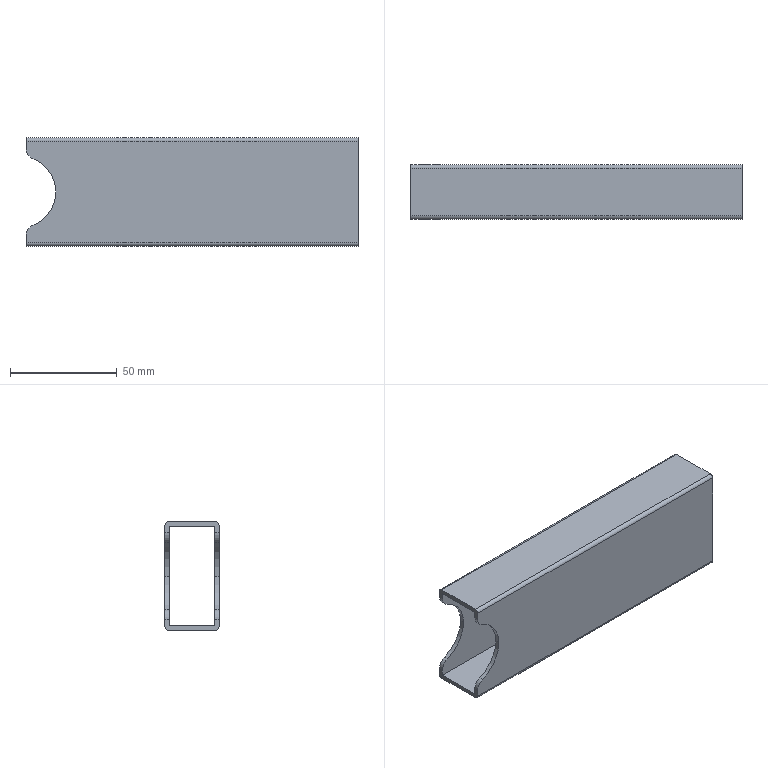Part | NX | features BREP 1 | 1 solid | 23 faces | box 155.702 x 25.4 x 50.8 mm | volume 42830 mm3 | cylinder 12 | plane 11 | commonest cylinder face diameters 3.175 x4 10.16 x4 33.528 x4
STEP:
#1=CARTESIAN_POINT('',(0.,12.7,-23.812));
#2=VERTEX_POINT('',#1);
#3=CARTESIAN_POINT('',(0.,12.7,-20.375));
#4=VERTEX_POINT('',#3);
#5=CARTESIAN_POINT('',(0.,12.7,-23.812));
#6=DIRECTION('',(0.,0.,1.));
#7=VECTOR('',#6,1000.);
#8=LINE('',#5,#7);
#9=EDGE_CURVE('',#2,#4,#8,.T.);
#10=ORIENTED_EDGE('',*,*,#9,.F.);
#11=CARTESIAN_POINT('',(0.,11.113,-25.4));
#12=VERTEX_POINT('',#11);
#13=CARTESIAN_POINT('',(0.,11.113,-23.812));
#14=DIRECTION('',(-1.,0.,0.));
#15=DIRECTION('',(0.,1.,0.));
#16=AXIS2_PLACEMENT_3D('',#13,#14,#15);
#17=CIRCLE('',#16,1.587);
#18=EDGE_CURVE('',#2,#12,#17,.T.);
#19=ORIENTED_EDGE('',*,*,#18,.T.);
#20=CARTESIAN_POINT('',(0.,-11.113,-25.4));
#21=VERTEX_POINT('',#20);
#22=CARTESIAN_POINT('',(0.,-11.113,-25.4));
#23=DIRECTION('',(0.,1.,0.));
#24=VECTOR('',#23,1000.);
#25=LINE('',#22,#24);
#26=EDGE_CURVE('',#21,#12,#25,.T.);
#27=ORIENTED_EDGE('',*,*,#26,.F.);
#28=CARTESIAN_POINT('',(0.,-12.7,-23.812));
#29=VERTEX_POINT('',#28);
#30=CARTESIAN_POINT('',(0.,-11.113,-23.812));
#31=DIRECTION('',(-1.,0.,0.));
#32=DIRECTION('',(0.,0.,-1.));
#33=AXIS2_PLACEMENT_3D('',#30,#31,#32);
#34=CIRCLE('',#33,1.587);
#35=EDGE_CURVE('',#21,#29,#34,.T.);
#36=ORIENTED_EDGE('',*,*,#35,.T.);
#37=CARTESIAN_POINT('',(0.,-12.7,-20.375));
#38=VERTEX_POINT('',#37);
#39=CARTESIAN_POINT('',(0.,-12.7,-20.375));
#40=DIRECTION('',(0.,0.,-1.));
#41=VECTOR('',#40,1000.);
#42=LINE('',#39,#41);
#43=EDGE_CURVE('',#38,#29,#42,.T.);
#44=ORIENTED_EDGE('',*,*,#43,.F.);
#45=CARTESIAN_POINT('',(0.,-10.719,-20.375));
#46=VERTEX_POINT('',#45);
#47=CARTESIAN_POINT('',(0.,-12.7,-20.375));
#48=DIRECTION('',(0.,1.,0.));
#49=VECTOR('',#48,1000.);
#50=LINE('',#47,#49);
#51=EDGE_CURVE('',#38,#46,#50,.T.);
#52=ORIENTED_EDGE('',*,*,#51,.T.);
#53=CARTESIAN_POINT('',(0.,-10.719,-23.419));
#54=VERTEX_POINT('',#53);
#55=CARTESIAN_POINT('',(0.,-10.719,-23.419));
#56=DIRECTION('',(0.,0.,1.));
#57=VECTOR('',#56,1000.);
#58=LINE('',#55,#57);
#59=EDGE_CURVE('',#54,#46,#58,.T.);
#60=ORIENTED_EDGE('',*,*,#59,.F.);
#61=CARTESIAN_POINT('',(0.,10.719,-23.419));
#62=VERTEX_POINT('',#61);
#63=CARTESIAN_POINT('',(0.,10.719,-23.419));
#64=DIRECTION('',(0.,-1.,0.));
#65=VECTOR('',#64,1000.);
#66=LINE('',#63,#65);
#67=EDGE_CURVE('',#62,#54,#66,.T.);
#68=ORIENTED_EDGE('',*,*,#67,.F.);
#69=CARTESIAN_POINT('',(0.,10.719,-20.375));
#70=VERTEX_POINT('',#69);
#71=CARTESIAN_POINT('',(0.,10.719,-20.375));
#72=DIRECTION('',(0.,0.,-1.));
#73=VECTOR('',#72,1000.);
#74=LINE('',#71,#73);
#75=EDGE_CURVE('',#70,#62,#74,.T.);
#76=ORIENTED_EDGE('',*,*,#75,.F.);
#77=CARTESIAN_POINT('',(0.,10.719,-20.375));
#78=DIRECTION('',(0.,1.,0.));
#79=VECTOR('',#78,1000.);
#80=LINE('',#77,#79);
#81=EDGE_CURVE('',#70,#4,#80,.T.);
#82=ORIENTED_EDGE('',*,*,#81,.T.);
#83=EDGE_LOOP('',(#10,#19,#27,#36,#44,#52,#60,#68,#76,#82));
#84=FACE_BOUND('',#83,.T.);
#85=CARTESIAN_POINT('',(0.,0.,0.));
#86=DIRECTION('',(1.,0.,0.));
#87=DIRECTION('',(0.,1.,0.));
#88=AXIS2_PLACEMENT_3D('',#85,#86,#87);
#89=PLANE('',#88);
#90=ADVANCED_FACE('',(#84),#89,.F.);
#91=CARTESIAN_POINT('',(0.,-12.7,23.812));
#92=VERTEX_POINT('',#91);
#93=CARTESIAN_POINT('',(0.,-12.7,20.375));
#94=VERTEX_POINT('',#93);
#95=CARTESIAN_POINT('',(0.,-12.7,23.812));
#96=DIRECTION('',(0.,0.,-1.));
#97=VECTOR('',#96,1000.);
#98=LINE('',#95,#97);
#99=EDGE_CURVE('',#92,#94,#98,.T.);
#100=ORIENTED_EDGE('',*,*,#99,.F.);
#101=CARTESIAN_POINT('',(0.,-11.113,25.4));
#102=VERTEX_POINT('',#101);
#103=CARTESIAN_POINT('',(0.,-11.113,23.812));
#104=DIRECTION('',(-1.,0.,0.));
#105=DIRECTION('',(0.,-1.,0.));
#106=AXIS2_PLACEMENT_3D('',#103,#104,#105);
#107=CIRCLE('',#106,1.587);
#108=EDGE_CURVE('',#92,#102,#107,.T.);
#109=ORIENTED_EDGE('',*,*,#108,.T.);
#110=CARTESIAN_POINT('',(0.,11.113,25.4));
#111=VERTEX_POINT('',#110);
#112=CARTESIAN_POINT('',(0.,11.113,25.4));
#113=DIRECTION('',(0.,-1.,0.));
#114=VECTOR('',#113,1000.);
#115=LINE('',#112,#114);
#116=EDGE_CURVE('',#111,#102,#115,.T.);
#117=ORIENTED_EDGE('',*,*,#116,.F.);
#118=CARTESIAN_POINT('',(0.,12.7,23.812));
#119=VERTEX_POINT('',#118);
#120=CARTESIAN_POINT('',(0.,11.113,23.812));
#121=DIRECTION('',(-1.,0.,0.));
#122=DIRECTION('',(0.,0.,1.));
#123=AXIS2_PLACEMENT_3D('',#120,#121,#122);
#124=CIRCLE('',#123,1.587);
#125=EDGE_CURVE('',#111,#119,#124,.T.);
#126=ORIENTED_EDGE('',*,*,#125,.T.);
#127=CARTESIAN_POINT('',(0.,12.7,20.375));
#128=VERTEX_POINT('',#127);
#129=CARTESIAN_POINT('',(0.,12.7,20.375));
#130=DIRECTION('',(0.,0.,1.));
#131=VECTOR('',#130,1000.);
#132=LINE('',#129,#131);
#133=EDGE_CURVE('',#128,#119,#132,.T.);
#134=ORIENTED_EDGE('',*,*,#133,.F.);
#135=CARTESIAN_POINT('',(0.,10.719,20.375));
#136=VERTEX_POINT('',#135);
#137=CARTESIAN_POINT('',(0.,12.7,20.375));
#138=DIRECTION('',(0.,-1.,0.));
#139=VECTOR('',#138,1000.);
#140=LINE('',#137,#139);
#141=EDGE_CURVE('',#128,#136,#140,.T.);
#142=ORIENTED_EDGE('',*,*,#141,.T.);
#143=CARTESIAN_POINT('',(0.,10.719,23.419));
#144=VERTEX_POINT('',#143);
#145=CARTESIAN_POINT('',(0.,10.719,23.419));
#146=DIRECTION('',(0.,0.,-1.));
#147=VECTOR('',#146,1000.);
#148=LINE('',#145,#147);
#149=EDGE_CURVE('',#144,#136,#148,.T.);
#150=ORIENTED_EDGE('',*,*,#149,.F.);
#151=CARTESIAN_POINT('',(0.,-10.719,23.419));
#152=VERTEX_POINT('',#151);
#153=CARTESIAN_POINT('',(0.,-10.719,23.419));
#154=DIRECTION('',(0.,1.,0.));
#155=VECTOR('',#154,1000.);
#156=LINE('',#153,#155);
#157=EDGE_CURVE('',#152,#144,#156,.T.);
#158=ORIENTED_EDGE('',*,*,#157,.F.);
#159=CARTESIAN_POINT('',(0.,-10.719,20.375));
#160=VERTEX_POINT('',#159);
#161=CARTESIAN_POINT('',(0.,-10.719,20.375));
#162=DIRECTION('',(0.,0.,1.));
#163=VECTOR('',#162,1000.);
#164=LINE('',#161,#163);
#165=EDGE_CURVE('',#160,#152,#164,.T.);
#166=ORIENTED_EDGE('',*,*,#165,.F.);
#167=CARTESIAN_POINT('',(0.,-10.719,20.375));
#168=DIRECTION('',(0.,-1.,0.));
#169=VECTOR('',#168,1000.);
#170=LINE('',#167,#169);
#171=EDGE_CURVE('',#160,#94,#170,.T.);
#172=ORIENTED_EDGE('',*,*,#171,.T.);
#173=EDGE_LOOP('',(#100,#109,#117,#126,#134,#142,#150,#158,#166,#172));
#174=FACE_BOUND('',#173,.T.);
#175=CARTESIAN_POINT('',(0.,0.,0.));
#176=DIRECTION('',(1.,0.,0.));
#177=DIRECTION('',(0.,1.,0.));
#178=AXIS2_PLACEMENT_3D('',#175,#176,#177);
#179=PLANE('',#178);
#180=ADVANCED_FACE('',(#174),#179,.F.);
#181=CARTESIAN_POINT('',(3.249,10.719,-15.637));
#182=VERTEX_POINT('',#181);
#183=CARTESIAN_POINT('',(5.08,10.719,-20.375));
#184=DIRECTION('',(0.,-1.,0.));
#185=DIRECTION('',(-0.3605,0.,0.9328));
#186=AXIS2_PLACEMENT_3D('',#183,#184,#185);
#187=CIRCLE('',#186,5.08);
#188=EDGE_CURVE('',#182,#70,#187,.T.);
#189=ORIENTED_EDGE('',*,*,#188,.F.);
#190=CARTESIAN_POINT('',(3.249,12.7,-15.637));
#191=VERTEX_POINT('',#190);
#192=CARTESIAN_POINT('',(3.249,10.719,-15.637));
#193=DIRECTION('',(0.,1.,0.));
#194=VECTOR('',#193,1000.);
#195=LINE('',#192,#194);
#196=EDGE_CURVE('',#182,#191,#195,.T.);
#197=ORIENTED_EDGE('',*,*,#196,.T.);
#198=CARTESIAN_POINT('',(5.08,12.7,-20.375));
#199=DIRECTION('',(0.,1.,0.));
#200=DIRECTION('',(-1.,0.,0.));
#201=AXIS2_PLACEMENT_3D('',#198,#199,#200);
#202=CIRCLE('',#201,5.08);
#203=EDGE_CURVE('',#4,#191,#202,.T.);
#204=ORIENTED_EDGE('',*,*,#203,.F.);
#205=ORIENTED_EDGE('',*,*,#81,.F.);
#206=EDGE_LOOP('',(#189,#197,#204,#205));
#207=FACE_BOUND('',#206,.T.);
#208=CARTESIAN_POINT('',(5.08,-12.922,-20.375));
#209=DIRECTION('',(0.,1.,0.));
#210=DIRECTION('',(-1.,0.,0.));
#211=AXIS2_PLACEMENT_3D('',#208,#209,#210);
#212=CYLINDRICAL_SURFACE('',#211,5.08);
#213=ADVANCED_FACE('',(#207),#212,.T.);
#214=CARTESIAN_POINT('',(3.249,12.7,15.637));
#215=VERTEX_POINT('',#214);
#216=CARTESIAN_POINT('',(13.97,12.7,0.));
#217=VERTEX_POINT('',#216);
#218=CARTESIAN_POINT('',(-2.794,12.7,0.));
#219=DIRECTION('',(0.,1.,0.));
#220=DIRECTION('',(0.3605,0.,0.9328));
#221=AXIS2_PLACEMENT_3D('',#218,#219,#220);
#222=CIRCLE('',#221,16.764);
#223=EDGE_CURVE('',#215,#217,#222,.T.);
#224=ORIENTED_EDGE('',*,*,#223,.F.);
#225=CARTESIAN_POINT('',(5.08,12.7,20.375));
#226=DIRECTION('',(0.,1.,0.));
#227=DIRECTION('',(-0.3605,0.,-0.9328));
#228=AXIS2_PLACEMENT_3D('',#225,#226,#227);
#229=CIRCLE('',#228,5.08);
#230=EDGE_CURVE('',#215,#128,#229,.T.);
#231=ORIENTED_EDGE('',*,*,#230,.T.);
#232=ORIENTED_EDGE('',*,*,#133,.T.);
#233=CARTESIAN_POINT('',(155.702,12.7,23.812));
#234=VERTEX_POINT('',#233);
#235=CARTESIAN_POINT('',(155.702,12.7,23.812));
#236=DIRECTION('',(-1.,0.,0.));
#237=VECTOR('',#236,1000.);
#238=LINE('',#235,#237);
#239=EDGE_CURVE('',#234,#119,#238,.T.);
#240=ORIENTED_EDGE('',*,*,#239,.F.);
#241=CARTESIAN_POINT('',(155.702,12.7,-23.812));
#242=VERTEX_POINT('',#241);
#243=CARTESIAN_POINT('',(155.702,12.7,-23.812));
#244=DIRECTION('',(0.,0.,1.));
#245=VECTOR('',#244,1000.);
#246=LINE('',#243,#245);
#247=EDGE_CURVE('',#242,#234,#246,.T.);
#248=ORIENTED_EDGE('',*,*,#247,.F.);
#249=CARTESIAN_POINT('',(155.702,12.7,-23.812));
#250=DIRECTION('',(-1.,0.,0.));
#251=VECTOR('',#250,1000.);
#252=LINE('',#249,#251);
#253=EDGE_CURVE('',#242,#2,#252,.T.);
#254=ORIENTED_EDGE('',*,*,#253,.T.);
#255=ORIENTED_EDGE('',*,*,#9,.T.);
#256=ORIENTED_EDGE('',*,*,#203,.T.);
#257=CARTESIAN_POINT('',(-2.794,12.7,0.));
#258=DIRECTION('',(0.,1.,0.));
#259=DIRECTION('',(0.3605,0.,0.9328));
#260=AXIS2_PLACEMENT_3D('',#257,#258,#259);
#261=CIRCLE('',#260,16.764);
#262=EDGE_CURVE('',#217,#191,#261,.T.);
#263=ORIENTED_EDGE('',*,*,#262,.F.);
#264=EDGE_LOOP('',(#224,#231,#232,#240,#248,#254,#255,#256,#263));
#265=FACE_BOUND('',#264,.T.);
#266=CARTESIAN_POINT('',(0.,12.7,-25.4));
#267=DIRECTION('',(0.,1.,0.));
#268=DIRECTION('',(1.,0.,0.));
#269=AXIS2_PLACEMENT_3D('',#266,#267,#268);
#270=PLANE('',#269);
#271=ADVANCED_FACE('',(#265),#270,.T.);
#272=CARTESIAN_POINT('',(155.702,11.113,-25.4));
#273=VERTEX_POINT('',#272);
#274=CARTESIAN_POINT('',(155.702,11.113,-23.812));
#275=DIRECTION('',(1.,0.,0.));
#276=DIRECTION('',(0.,0.,-1.));
#277=AXIS2_PLACEMENT_3D('',#274,#275,#276);
#278=CIRCLE('',#277,1.587);
#279=EDGE_CURVE('',#273,#242,#278,.T.);
#280=ORIENTED_EDGE('',*,*,#279,.F.);
#281=CARTESIAN_POINT('',(155.702,11.113,-25.4));
#282=DIRECTION('',(-1.,0.,0.));
#283=VECTOR('',#282,1000.);
#284=LINE('',#281,#283);
#285=EDGE_CURVE('',#273,#12,#284,.T.);
#286=ORIENTED_EDGE('',*,*,#285,.T.);
#287=ORIENTED_EDGE('',*,*,#18,.F.);
#288=ORIENTED_EDGE('',*,*,#253,.F.);
#289=EDGE_LOOP('',(#280,#286,#287,#288));
#290=FACE_BOUND('',#289,.T.);
#291=CARTESIAN_POINT('',(155.961,11.113,-23.812));
#292=DIRECTION('',(-1.,0.,0.));
#293=DIRECTION('',(0.,1.,0.));
#294=AXIS2_PLACEMENT_3D('',#291,#292,#293);
#295=CYLINDRICAL_SURFACE('',#294,1.587);
#296=ADVANCED_FACE('',(#290),#295,.T.);
#297=CARTESIAN_POINT('',(155.702,-11.113,-25.4));
#298=VERTEX_POINT('',#297);
#299=CARTESIAN_POINT('',(155.702,-11.113,-25.4));
#300=DIRECTION('',(0.,1.,0.));
#301=VECTOR('',#300,1000.);
#302=LINE('',#299,#301);
#303=EDGE_CURVE('',#298,#273,#302,.T.);
#304=ORIENTED_EDGE('',*,*,#303,.F.);
#305=CARTESIAN_POINT('',(155.702,-11.113,-25.4));
#306=DIRECTION('',(-1.,0.,0.));
#307=VECTOR('',#306,1000.);
#308=LINE('',#305,#307);
#309=EDGE_CURVE('',#298,#21,#308,.T.);
#310=ORIENTED_EDGE('',*,*,#309,.T.);
#311=ORIENTED_EDGE('',*,*,#26,.T.);
#312=ORIENTED_EDGE('',*,*,#285,.F.);
#313=EDGE_LOOP('',(#304,#310,#311,#312));
#314=FACE_BOUND('',#313,.T.);
#315=CARTESIAN_POINT('',(0.,-12.7,-25.4));
#316=DIRECTION('',(0.,0.,-1.));
#317=DIRECTION('',(0.,-1.,0.));
#318=AXIS2_PLACEMENT_3D('',#315,#316,#317);
#319=PLANE('',#318);
#320=ADVANCED_FACE('',(#314),#319,.T.);
#321=CARTESIAN_POINT('',(155.702,-12.7,-23.812));
#322=VERTEX_POINT('',#321);
#323=CARTESIAN_POINT('',(155.702,-11.113,-23.812));
#324=DIRECTION('',(1.,0.,0.));
#325=DIRECTION('',(0.,-1.,0.));
#326=AXIS2_PLACEMENT_3D('',#323,#324,#325);
#327=CIRCLE('',#326,1.587);
#328=EDGE_CURVE('',#322,#298,#327,.T.);
#329=ORIENTED_EDGE('',*,*,#328,.F.);
#330=CARTESIAN_POINT('',(155.702,-12.7,-23.812));
#331=DIRECTION('',(-1.,0.,0.));
#332=VECTOR('',#331,1000.);
#333=LINE('',#330,#332);
#334=EDGE_CURVE('',#322,#29,#333,.T.);
#335=ORIENTED_EDGE('',*,*,#334,.T.);
#336=ORIENTED_EDGE('',*,*,#35,.F.);
#337=ORIENTED_EDGE('',*,*,#309,.F.);
#338=EDGE_LOOP('',(#329,#335,#336,#337));
#339=FACE_BOUND('',#338,.T.);
#340=CARTESIAN_POINT('',(155.961,-11.113,-23.812));
#341=DIRECTION('',(-1.,0.,0.));
#342=DIRECTION('',(0.,0.,-1.));
#343=AXIS2_PLACEMENT_3D('',#340,#341,#342);
#344=CYLINDRICAL_SURFACE('',#343,1.587);
#345=ADVANCED_FACE('',(#339),#344,.T.);
#346=ORIENTED_EDGE('',*,*,#43,.T.);
#347=ORIENTED_EDGE('',*,*,#334,.F.);
#348=CARTESIAN_POINT('',(155.702,-12.7,23.812));
#349=VERTEX_POINT('',#348);
#350=CARTESIAN_POINT('',(155.702,-12.7,23.812));
#351=DIRECTION('',(0.,0.,-1.));
#352=VECTOR('',#351,1000.);
#353=LINE('',#350,#352);
#354=EDGE_CURVE('',#349,#322,#353,.T.);
#355=ORIENTED_EDGE('',*,*,#354,.F.);
#356=CARTESIAN_POINT('',(155.702,-12.7,23.812));
#357=DIRECTION('',(-1.,0.,0.));
#358=VECTOR('',#357,1000.);
#359=LINE('',#356,#358);
#360=EDGE_CURVE('',#349,#92,#359,.T.);
#361=ORIENTED_EDGE('',*,*,#360,.T.);
#362=ORIENTED_EDGE('',*,*,#99,.T.);
#363=CARTESIAN_POINT('',(3.249,-12.7,15.637));
#364=VERTEX_POINT('',#363);
#365=CARTESIAN_POINT('',(5.08,-12.7,20.375));
#366=DIRECTION('',(0.,-1.,0.));
#367=DIRECTION('',(-1.,0.,0.));
#368=AXIS2_PLACEMENT_3D('',#365,#366,#367);
#369=CIRCLE('',#368,5.08);
#370=EDGE_CURVE('',#94,#364,#369,.T.);
#371=ORIENTED_EDGE('',*,*,#370,.T.);
#372=CARTESIAN_POINT('',(13.97,-12.7,0.));
#373=VERTEX_POINT('',#372);
#374=CARTESIAN_POINT('',(-2.794,-12.7,0.));
#375=DIRECTION('',(0.,1.,0.));
#376=DIRECTION('',(0.3605,0.,0.9328));
#377=AXIS2_PLACEMENT_3D('',#374,#375,#376);
#378=CIRCLE('',#377,16.764);
#379=EDGE_CURVE('',#364,#373,#378,.T.);
#380=ORIENTED_EDGE('',*,*,#379,.T.);
#381=CARTESIAN_POINT('',(3.249,-12.7,-15.637));
#382=VERTEX_POINT('',#381);
#383=CARTESIAN_POINT('',(-2.794,-12.7,0.));
#384=DIRECTION('',(0.,1.,0.));
#385=DIRECTION('',(0.3605,0.,0.9328));
#386=AXIS2_PLACEMENT_3D('',#383,#384,#385);
#387=CIRCLE('',#386,16.764);
#388=EDGE_CURVE('',#373,#382,#387,.T.);
#389=ORIENTED_EDGE('',*,*,#388,.T.);
#390=CARTESIAN_POINT('',(5.08,-12.7,-20.375));
#391=DIRECTION('',(0.,-1.,0.));
#392=DIRECTION('',(-0.3605,0.,0.9328));
#393=AXIS2_PLACEMENT_3D('',#390,#391,#392);
#394=CIRCLE('',#393,5.08);
#395=EDGE_CURVE('',#382,#38,#394,.T.);
#396=ORIENTED_EDGE('',*,*,#395,.T.);
#397=EDGE_LOOP('',(#346,#347,#355,#361,#362,#371,#380,#389,#396));
#398=FACE_BOUND('',#397,.T.);
#399=CARTESIAN_POINT('',(0.,-12.7,25.4));
#400=DIRECTION('',(0.,-1.,0.));
#401=DIRECTION('',(0.,0.,-1.));
#402=AXIS2_PLACEMENT_3D('',#399,#400,#401);
#403=PLANE('',#402);
#404=ADVANCED_FACE('',(#398),#403,.T.);
#405=ORIENTED_EDGE('',*,*,#395,.F.);
#406=CARTESIAN_POINT('',(3.249,-10.719,-15.637));
#407=VERTEX_POINT('',#406);
#408=CARTESIAN_POINT('',(3.249,-12.7,-15.637));
#409=DIRECTION('',(0.,1.,0.));
#410=VECTOR('',#409,1000.);
#411=LINE('',#408,#410);
#412=EDGE_CURVE('',#382,#407,#411,.T.);
#413=ORIENTED_EDGE('',*,*,#412,.T.);
#414=CARTESIAN_POINT('',(5.08,-10.719,-20.375));
#415=DIRECTION('',(0.,1.,0.));
#416=DIRECTION('',(-1.,0.,0.));
#417=AXIS2_PLACEMENT_3D('',#414,#415,#416);
#418=CIRCLE('',#417,5.08);
#419=EDGE_CURVE('',#46,#407,#418,.T.);
#420=ORIENTED_EDGE('',*,*,#419,.F.);
#421=ORIENTED_EDGE('',*,*,#51,.F.);
#422=EDGE_LOOP('',(#405,#413,#420,#421));
#423=FACE_BOUND('',#422,.T.);
#424=CARTESIAN_POINT('',(5.08,-12.922,-20.375));
#425=DIRECTION('',(0.,1.,0.));
#426=DIRECTION('',(-1.,0.,0.));
#427=AXIS2_PLACEMENT_3D('',#424,#425,#426);
#428=CYLINDRICAL_SURFACE('',#427,5.08);
#429=ADVANCED_FACE('',(#423),#428,.T.);
#430=CARTESIAN_POINT('',(3.249,-10.719,15.637));
#431=VERTEX_POINT('',#430);
#432=CARTESIAN_POINT('',(13.97,-10.719,0.));
#433=VERTEX_POINT('',#432);
#434=CARTESIAN_POINT('',(-2.794,-10.719,0.));
#435=DIRECTION('',(0.,1.,0.));
#436=DIRECTION('',(0.3605,0.,0.9328));
#437=AXIS2_PLACEMENT_3D('',#434,#435,#436);
#438=CIRCLE('',#437,16.764);
#439=EDGE_CURVE('',#431,#433,#438,.T.);
#440=ORIENTED_EDGE('',*,*,#439,.F.);
#441=CARTESIAN_POINT('',(5.08,-10.719,20.375));
#442=DIRECTION('',(0.,1.,0.));
#443=DIRECTION('',(-0.3605,0.,-0.9328));
#444=AXIS2_PLACEMENT_3D('',#441,#442,#443);
#445=CIRCLE('',#444,5.08);
#446=EDGE_CURVE('',#431,#160,#445,.T.);
#447=ORIENTED_EDGE('',*,*,#446,.T.);
#448=ORIENTED_EDGE('',*,*,#165,.T.);
#449=CARTESIAN_POINT('',(155.702,-10.719,23.419));
#450=VERTEX_POINT('',#449);
#451=CARTESIAN_POINT('',(0.,-10.719,23.419));
#452=DIRECTION('',(1.,0.,0.));
#453=VECTOR('',#452,1000.);
#454=LINE('',#451,#453);
#455=EDGE_CURVE('',#152,#450,#454,.T.);
#456=ORIENTED_EDGE('',*,*,#455,.T.);
#457=CARTESIAN_POINT('',(155.702,-10.719,-23.419));
#458=VERTEX_POINT('',#457);
#459=CARTESIAN_POINT('',(155.702,-10.719,-23.419));
#460=DIRECTION('',(0.,0.,1.));
#461=VECTOR('',#460,1000.);
#462=LINE('',#459,#461);
#463=EDGE_CURVE('',#458,#450,#462,.T.);
#464=ORIENTED_EDGE('',*,*,#463,.F.);
#465=CARTESIAN_POINT('',(0.,-10.719,-23.419));
#466=DIRECTION('',(1.,0.,0.));
#467=VECTOR('',#466,1000.);
#468=LINE('',#465,#467);
#469=EDGE_CURVE('',#54,#458,#468,.T.);
#470=ORIENTED_EDGE('',*,*,#469,.F.);
#471=ORIENTED_EDGE('',*,*,#59,.T.);
#472=ORIENTED_EDGE('',*,*,#419,.T.);
#473=CARTESIAN_POINT('',(-2.794,-10.719,0.));
#474=DIRECTION('',(0.,1.,0.));
#475=DIRECTION('',(0.3605,0.,0.9328));
#476=AXIS2_PLACEMENT_3D('',#473,#474,#475);
#477=CIRCLE('',#476,16.764);
#478=EDGE_CURVE('',#433,#407,#477,.T.);
#479=ORIENTED_EDGE('',*,*,#478,.F.);
#480=EDGE_LOOP('',(#440,#447,#448,#456,#464,#470,#471,#472,#479));
#481=FACE_BOUND('',#480,.T.);
#482=CARTESIAN_POINT('',(0.,-10.719,-23.419));
#483=DIRECTION('',(0.,1.,0.));
#484=DIRECTION('',(1.,0.,0.));
#485=AXIS2_PLACEMENT_3D('',#482,#483,#484);
#486=PLANE('',#485);
#487=ADVANCED_FACE('',(#481),#486,.T.);
#488=ORIENTED_EDGE('',*,*,#469,.T.);
#489=CARTESIAN_POINT('',(155.702,10.719,-23.419));
#490=VERTEX_POINT('',#489);
#491=CARTESIAN_POINT('',(155.702,10.719,-23.419));
#492=DIRECTION('',(0.,-1.,0.));
#493=VECTOR('',#492,1000.);
#494=LINE('',#491,#493);
#495=EDGE_CURVE('',#490,#458,#494,.T.);
#496=ORIENTED_EDGE('',*,*,#495,.F.);
#497=CARTESIAN_POINT('',(0.,10.719,-23.419));
#498=DIRECTION('',(1.,0.,0.));
#499=VECTOR('',#498,1000.);
#500=LINE('',#497,#499);
#501=EDGE_CURVE('',#62,#490,#500,.T.);
#502=ORIENTED_EDGE('',*,*,#501,.F.);
#503=ORIENTED_EDGE('',*,*,#67,.T.);
#504=EDGE_LOOP('',(#488,#496,#502,#503));
#505=FACE_BOUND('',#504,.T.);
#506=CARTESIAN_POINT('',(0.,10.719,-23.419));
#507=DIRECTION('',(0.,0.,1.));
#508=DIRECTION('',(1.,0.,0.));
#509=AXIS2_PLACEMENT_3D('',#506,#507,#508);
#510=PLANE('',#509);
#511=ADVANCED_FACE('',(#505),#510,.T.);
#512=ORIENTED_EDGE('',*,*,#75,.T.);
#513=ORIENTED_EDGE('',*,*,#501,.T.);
#514=CARTESIAN_POINT('',(155.702,10.719,23.419));
#515=VERTEX_POINT('',#514);
#516=CARTESIAN_POINT('',(155.702,10.719,23.419));
#517=DIRECTION('',(0.,0.,-1.));
#518=VECTOR('',#517,1000.);
#519=LINE('',#516,#518);
#520=EDGE_CURVE('',#515,#490,#519,.T.);
#521=ORIENTED_EDGE('',*,*,#520,.F.);
#522=CARTESIAN_POINT('',(0.,10.719,23.419));
#523=DIRECTION('',(1.,0.,0.));
#524=VECTOR('',#523,1000.);
#525=LINE('',#522,#524);
#526=EDGE_CURVE('',#144,#515,#525,.T.);
#527=ORIENTED_EDGE('',*,*,#526,.F.);
#528=ORIENTED_EDGE('',*,*,#149,.T.);
#529=CARTESIAN_POINT('',(3.249,10.719,15.637));
#530=VERTEX_POINT('',#529);
#531=CARTESIAN_POINT('',(5.08,10.719,20.375));
#532=DIRECTION('',(0.,-1.,0.));
#533=DIRECTION('',(-1.,0.,0.));
#534=AXIS2_PLACEMENT_3D('',#531,#532,#533);
#535=CIRCLE('',#534,5.08);
#536=EDGE_CURVE('',#136,#530,#535,.T.);
#537=ORIENTED_EDGE('',*,*,#536,.T.);
#538=CARTESIAN_POINT('',(13.97,10.719,0.));
#539=VERTEX_POINT('',#538);
#540=CARTESIAN_POINT('',(-2.794,10.719,0.));
#541=DIRECTION('',(0.,1.,0.));
#542=DIRECTION('',(0.3605,0.,0.9328));
#543=AXIS2_PLACEMENT_3D('',#540,#541,#542);
#544=CIRCLE('',#543,16.764);
#545=EDGE_CURVE('',#530,#539,#544,.T.);
#546=ORIENTED_EDGE('',*,*,#545,.T.);
#547=CARTESIAN_POINT('',(-2.794,10.719,0.));
#548=DIRECTION('',(0.,1.,0.));
#549=DIRECTION('',(0.3605,0.,0.9328));
#550=AXIS2_PLACEMENT_3D('',#547,#548,#549);
#551=CIRCLE('',#550,16.764);
#552=EDGE_CURVE('',#539,#182,#551,.T.);
#553=ORIENTED_EDGE('',*,*,#552,.T.);
#554=ORIENTED_EDGE('',*,*,#188,.T.);
#555=EDGE_LOOP('',(#512,#513,#521,#527,#528,#537,#546,#553,#554));
#556=FACE_BOUND('',#555,.T.);
#557=CARTESIAN_POINT('',(0.,10.719,23.419));
#558=DIRECTION('',(0.,-1.,0.));
#559=DIRECTION('',(0.,0.,-1.));
#560=AXIS2_PLACEMENT_3D('',#557,#558,#559);
#561=PLANE('',#560);
#562=ADVANCED_FACE('',(#556),#561,.T.);
#563=CARTESIAN_POINT('',(13.97,15.24,0.));
#564=DIRECTION('',(0.,1.,0.));
#565=VECTOR('',#564,1000.);
#566=LINE('',#563,#565);
#567=EDGE_CURVE('',#539,#217,#566,.T.);
#568=ORIENTED_EDGE('',*,*,#567,.F.);
#569=ORIENTED_EDGE('',*,*,#545,.F.);
#570=CARTESIAN_POINT('',(3.249,12.7,15.637));
#571=DIRECTION('',(0.,-1.,0.));
#572=VECTOR('',#571,1000.);
#573=LINE('',#570,#572);
#574=EDGE_CURVE('',#215,#530,#573,.T.);
#575=ORIENTED_EDGE('',*,*,#574,.F.);
#576=ORIENTED_EDGE('',*,*,#223,.T.);
#577=EDGE_LOOP('',(#568,#569,#575,#576));
#578=FACE_BOUND('',#577,.T.);
#579=CARTESIAN_POINT('',(-2.794,15.24,0.));
#580=DIRECTION('',(0.,1.,0.));
#581=DIRECTION('',(1.,0.,0.));
#582=AXIS2_PLACEMENT_3D('',#579,#580,#581);
#583=CYLINDRICAL_SURFACE('',#582,16.764);
#584=ADVANCED_FACE('',(#578),#583,.F.);
#585=CARTESIAN_POINT('',(13.97,15.24,0.));
#586=DIRECTION('',(0.,1.,0.));
#587=VECTOR('',#586,1000.);
#588=LINE('',#585,#587);
#589=EDGE_CURVE('',#373,#433,#588,.T.);
#590=ORIENTED_EDGE('',*,*,#589,.F.);
#591=ORIENTED_EDGE('',*,*,#379,.F.);
#592=CARTESIAN_POINT('',(3.249,-10.719,15.637));
#593=DIRECTION('',(0.,-1.,0.));
#594=VECTOR('',#593,1000.);
#595=LINE('',#592,#594);
#596=EDGE_CURVE('',#431,#364,#595,.T.);
#597=ORIENTED_EDGE('',*,*,#596,.F.);
#598=ORIENTED_EDGE('',*,*,#439,.T.);
#599=EDGE_LOOP('',(#590,#591,#597,#598));
#600=FACE_BOUND('',#599,.T.);
#601=CARTESIAN_POINT('',(-2.794,15.24,0.));
#602=DIRECTION('',(0.,1.,0.));
#603=DIRECTION('',(1.,0.,0.));
#604=AXIS2_PLACEMENT_3D('',#601,#602,#603);
#605=CYLINDRICAL_SURFACE('',#604,16.764);
#606=ADVANCED_FACE('',(#600),#605,.F.);
#607=ORIENTED_EDGE('',*,*,#230,.F.);
#608=ORIENTED_EDGE('',*,*,#574,.T.);
#609=ORIENTED_EDGE('',*,*,#536,.F.);
#610=ORIENTED_EDGE('',*,*,#141,.F.);
#611=EDGE_LOOP('',(#607,#608,#609,#610));
#612=FACE_BOUND('',#611,.T.);
#613=CARTESIAN_POINT('',(5.08,12.967,20.375));
#614=DIRECTION('',(0.,-1.,0.));
#615=DIRECTION('',(-1.,0.,0.));
#616=AXIS2_PLACEMENT_3D('',#613,#614,#615);
#617=CYLINDRICAL_SURFACE('',#616,5.08);
#618=ADVANCED_FACE('',(#612),#617,.T.);
#619=ORIENTED_EDGE('',*,*,#446,.F.);
#620=ORIENTED_EDGE('',*,*,#596,.T.);
#621=ORIENTED_EDGE('',*,*,#370,.F.);
#622=ORIENTED_EDGE('',*,*,#171,.F.);
#623=EDGE_LOOP('',(#619,#620,#621,#622));
#624=FACE_BOUND('',#623,.T.);
#625=CARTESIAN_POINT('',(5.08,12.967,20.375));
#626=DIRECTION('',(0.,-1.,0.));
#627=DIRECTION('',(-1.,0.,0.));
#628=AXIS2_PLACEMENT_3D('',#625,#626,#627);
#629=CYLINDRICAL_SURFACE('',#628,5.08);
#630=ADVANCED_FACE('',(#624),#629,.T.);
#631=ORIENTED_EDGE('',*,*,#526,.T.);
#632=CARTESIAN_POINT('',(155.702,-10.719,23.419));
#633=DIRECTION('',(0.,1.,0.));
#634=VECTOR('',#633,1000.);
#635=LINE('',#632,#634);
#636=EDGE_CURVE('',#450,#515,#635,.T.);
#637=ORIENTED_EDGE('',*,*,#636,.F.);
#638=ORIENTED_EDGE('',*,*,#455,.F.);
#639=ORIENTED_EDGE('',*,*,#157,.T.);
#640=EDGE_LOOP('',(#631,#637,#638,#639));
#641=FACE_BOUND('',#640,.T.);
#642=CARTESIAN_POINT('',(0.,-10.719,23.419));
#643=DIRECTION('',(0.,0.,-1.));
#644=DIRECTION('',(0.,-1.,0.));
#645=AXIS2_PLACEMENT_3D('',#642,#643,#644);
#646=PLANE('',#645);
#647=ADVANCED_FACE('',(#641),#646,.T.);
#648=CARTESIAN_POINT('',(155.702,11.113,25.4));
#649=VERTEX_POINT('',#648);
#650=CARTESIAN_POINT('',(155.702,-11.113,25.4));
#651=VERTEX_POINT('',#650);
#652=CARTESIAN_POINT('',(155.702,11.113,25.4));
#653=DIRECTION('',(0.,-1.,0.));
#654=VECTOR('',#653,1000.);
#655=LINE('',#652,#654);
#656=EDGE_CURVE('',#649,#651,#655,.T.);
#657=ORIENTED_EDGE('',*,*,#656,.T.);
#658=CARTESIAN_POINT('',(155.702,-11.113,23.812));
#659=DIRECTION('',(1.,0.,0.));
#660=DIRECTION('',(0.,0.,1.));
#661=AXIS2_PLACEMENT_3D('',#658,#659,#660);
#662=CIRCLE('',#661,1.587);
#663=EDGE_CURVE('',#651,#349,#662,.T.);
#664=ORIENTED_EDGE('',*,*,#663,.T.);
#665=ORIENTED_EDGE('',*,*,#354,.T.);
#666=ORIENTED_EDGE('',*,*,#328,.T.);
#667=ORIENTED_EDGE('',*,*,#303,.T.);
#668=ORIENTED_EDGE('',*,*,#279,.T.);
#669=ORIENTED_EDGE('',*,*,#247,.T.);
#670=CARTESIAN_POINT('',(155.702,11.113,23.812));
#671=DIRECTION('',(1.,0.,0.));
#672=DIRECTION('',(0.,1.,0.));
#673=AXIS2_PLACEMENT_3D('',#670,#671,#672);
#674=CIRCLE('',#673,1.587);
#675=EDGE_CURVE('',#234,#649,#674,.T.);
#676=ORIENTED_EDGE('',*,*,#675,.T.);
#677=EDGE_LOOP('',(#657,#664,#665,#666,#667,#668,#669,#676));
#678=FACE_BOUND('',#677,.T.);
#679=ORIENTED_EDGE('',*,*,#463,.T.);
#680=ORIENTED_EDGE('',*,*,#636,.T.);
#681=ORIENTED_EDGE('',*,*,#520,.T.);
#682=ORIENTED_EDGE('',*,*,#495,.T.);
#683=EDGE_LOOP('',(#679,#680,#681,#682));
#684=FACE_BOUND('',#683,.T.);
#685=CARTESIAN_POINT('',(155.702,0.,0.));
#686=DIRECTION('',(1.,0.,0.));
#687=DIRECTION('',(0.,1.,0.));
#688=AXIS2_PLACEMENT_3D('',#685,#686,#687);
#689=PLANE('',#688);
#690=ADVANCED_FACE('',(#678,#684),#689,.T.);
#691=ORIENTED_EDGE('',*,*,#675,.F.);
#692=ORIENTED_EDGE('',*,*,#239,.T.);
#693=ORIENTED_EDGE('',*,*,#125,.F.);
#694=CARTESIAN_POINT('',(155.702,11.113,25.4));
#695=DIRECTION('',(-1.,0.,0.));
#696=VECTOR('',#695,1000.);
#697=LINE('',#694,#696);
#698=EDGE_CURVE('',#649,#111,#697,.T.);
#699=ORIENTED_EDGE('',*,*,#698,.F.);
#700=EDGE_LOOP('',(#691,#692,#693,#699));
#701=FACE_BOUND('',#700,.T.);
#702=CARTESIAN_POINT('',(155.961,11.113,23.812));
#703=DIRECTION('',(-1.,0.,0.));
#704=DIRECTION('',(0.,0.,1.));
#705=AXIS2_PLACEMENT_3D('',#702,#703,#704);
#706=CYLINDRICAL_SURFACE('',#705,1.587);
#707=ADVANCED_FACE('',(#701),#706,.T.);
#708=ORIENTED_EDGE('',*,*,#116,.T.);
#709=CARTESIAN_POINT('',(155.702,-11.113,25.4));
#710=DIRECTION('',(-1.,0.,0.));
#711=VECTOR('',#710,1000.);
#712=LINE('',#709,#711);
#713=EDGE_CURVE('',#651,#102,#712,.T.);
#714=ORIENTED_EDGE('',*,*,#713,.F.);
#715=ORIENTED_EDGE('',*,*,#656,.F.);
#716=ORIENTED_EDGE('',*,*,#698,.T.);
#717=EDGE_LOOP('',(#708,#714,#715,#716));
#718=FACE_BOUND('',#717,.T.);
#719=CARTESIAN_POINT('',(0.,12.7,25.4));
#720=DIRECTION('',(0.,0.,1.));
#721=DIRECTION('',(1.,0.,0.));
#722=AXIS2_PLACEMENT_3D('',#719,#720,#721);
#723=PLANE('',#722);
#724=ADVANCED_FACE('',(#718),#723,.T.);
#725=ORIENTED_EDGE('',*,*,#663,.F.);
#726=ORIENTED_EDGE('',*,*,#713,.T.);
#727=ORIENTED_EDGE('',*,*,#108,.F.);
#728=ORIENTED_EDGE('',*,*,#360,.F.);
#729=EDGE_LOOP('',(#725,#726,#727,#728));
#730=FACE_BOUND('',#729,.T.);
#731=CARTESIAN_POINT('',(155.961,-11.113,23.812));
#732=DIRECTION('',(-1.,0.,0.));
#733=DIRECTION('',(0.,-1.,0.));
#734=AXIS2_PLACEMENT_3D('',#731,#732,#733);
#735=CYLINDRICAL_SURFACE('',#734,1.587);
#736=ADVANCED_FACE('',(#730),#735,.T.);
#737=ORIENTED_EDGE('',*,*,#388,.F.);
#738=ORIENTED_EDGE('',*,*,#589,.T.);
#739=ORIENTED_EDGE('',*,*,#478,.T.);
#740=ORIENTED_EDGE('',*,*,#412,.F.);
#741=EDGE_LOOP('',(#737,#738,#739,#740));
#742=FACE_BOUND('',#741,.T.);
#743=CARTESIAN_POINT('',(-2.794,15.24,0.));
#744=DIRECTION('',(0.,1.,0.));
#745=DIRECTION('',(1.,0.,0.));
#746=AXIS2_PLACEMENT_3D('',#743,#744,#745);
#747=CYLINDRICAL_SURFACE('',#746,16.764);
#748=ADVANCED_FACE('',(#742),#747,.F.);
#749=ORIENTED_EDGE('',*,*,#552,.F.);
#750=ORIENTED_EDGE('',*,*,#567,.T.);
#751=ORIENTED_EDGE('',*,*,#262,.T.);
#752=ORIENTED_EDGE('',*,*,#196,.F.);
#753=EDGE_LOOP('',(#749,#750,#751,#752));
#754=FACE_BOUND('',#753,.T.);
#755=CARTESIAN_POINT('',(-2.794,15.24,0.));
#756=DIRECTION('',(0.,1.,0.));
#757=DIRECTION('',(1.,0.,0.));
#758=AXIS2_PLACEMENT_3D('',#755,#756,#757);
#759=CYLINDRICAL_SURFACE('',#758,16.764);
#760=ADVANCED_FACE('',(#754),#759,.F.);
#761=CLOSED_SHELL('',(#90,#180,#213,#271,#296,#320,#345,#404,#429,#487,#511,#562,#584,#606,#618,#630,#647,#690,#707,#724,#736,#748,#760));
#762=MANIFOLD_SOLID_BREP('',#761);
#763=(LENGTH_UNIT()NAMED_UNIT(*)SI_UNIT(.MILLI.,.METRE.));
#764=UNCERTAINTY_MEASURE_WITH_UNIT(LENGTH_MEASURE(0.00001),#763,'','');
#765=(NAMED_UNIT(*)PLANE_ANGLE_UNIT()SI_UNIT($,.RADIAN.));
#766=(NAMED_UNIT(*)SI_UNIT($,.STERADIAN.)SOLID_ANGLE_UNIT());
#767=(GEOMETRIC_REPRESENTATION_CONTEXT(3)GLOBAL_UNCERTAINTY_ASSIGNED_CONTEXT((#764))GLOBAL_UNIT_ASSIGNED_CONTEXT((#763,#765,#766))REPRESENTATION_CONTEXT('',''));
#768=ADVANCED_BREP_SHAPE_REPRESENTATION('',(#762),#767);